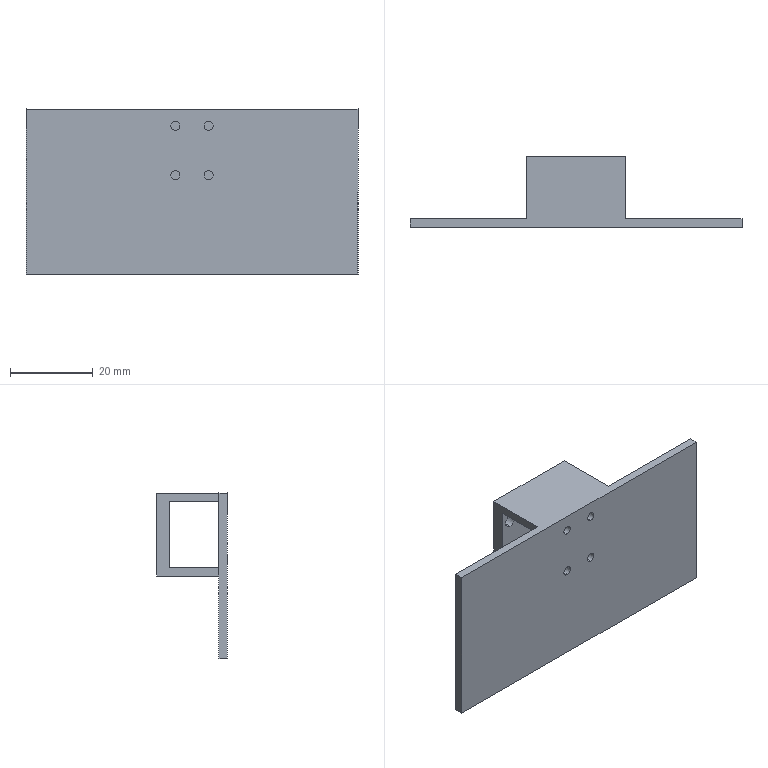Part | SolidWorks | features ICE 3, Extrusion 1 | 1 solid | 29 faces | box 80 x 17 x 40 mm | volume 8877 mm3 | cylinder 16 | plane 13 | commonest cylinder face diameters 2.2 x8 3 x8
STEP:
#1=CARTESIAN_POINT('',(9.5,14.,-3.));
#2=VERTEX_POINT('',#1);
#3=CARTESIAN_POINT('',(9.5,14.,-6.));
#4=VERTEX_POINT('',#3);
#5=CARTESIAN_POINT('',(9.5,14.,-4.5));
#6=DIRECTION('',(0.,-1.,0.));
#7=DIRECTION('',(0.,0.,-1.));
#8=AXIS2_PLACEMENT_3D('',#5,#6,#7);
#9=CIRCLE('',#8,1.5);
#10=EDGE_CURVE('',#2,#4,#9,.T.);
#11=ORIENTED_EDGE('',*,*,#10,.T.);
#12=CARTESIAN_POINT('',(9.5,17.,-6.));
#13=VERTEX_POINT('',#12);
#14=CARTESIAN_POINT('',(9.5,12.,-6.));
#15=DIRECTION('',(0.,1.,0.));
#16=VECTOR('',#15,1000.);
#17=LINE('',#14,#16);
#18=EDGE_CURVE('',#4,#13,#17,.T.);
#19=ORIENTED_EDGE('',*,*,#18,.T.);
#20=CARTESIAN_POINT('',(9.5,17.,-3.));
#21=VERTEX_POINT('',#20);
#22=CARTESIAN_POINT('',(9.5,17.,-4.5));
#23=DIRECTION('',(0.,1.,0.));
#24=DIRECTION('',(0.,0.,1.));
#25=AXIS2_PLACEMENT_3D('',#22,#23,#24);
#26=CIRCLE('',#25,1.5);
#27=EDGE_CURVE('',#13,#21,#26,.T.);
#28=ORIENTED_EDGE('',*,*,#27,.T.);
#29=CARTESIAN_POINT('',(9.5,12.,-3.));
#30=DIRECTION('',(0.,1.,0.));
#31=VECTOR('',#30,1000.);
#32=LINE('',#29,#31);
#33=EDGE_CURVE('',#2,#21,#32,.T.);
#34=ORIENTED_EDGE('',*,*,#33,.F.);
#35=EDGE_LOOP('',(#11,#19,#28,#34));
#36=FACE_OUTER_BOUND('',#35,.T.);
#37=CARTESIAN_POINT('',(9.5,12.,-4.5));
#38=DIRECTION('',(0.,1.,0.));
#39=DIRECTION('',(0.,0.,1.));
#40=AXIS2_PLACEMENT_3D('',#37,#38,#39);
#41=CYLINDRICAL_SURFACE('',#40,1.5);
#42=ADVANCED_FACE('',(#36),#41,.F.);
#43=CARTESIAN_POINT('',(-9.5,14.,-3.));
#44=VERTEX_POINT('',#43);
#45=CARTESIAN_POINT('',(-9.5,14.,-6.));
#46=VERTEX_POINT('',#45);
#47=CARTESIAN_POINT('',(-9.5,14.,-4.5));
#48=DIRECTION('',(0.,-1.,0.));
#49=DIRECTION('',(0.,0.,-1.));
#50=AXIS2_PLACEMENT_3D('',#47,#48,#49);
#51=CIRCLE('',#50,1.5);
#52=EDGE_CURVE('',#44,#46,#51,.T.);
#53=ORIENTED_EDGE('',*,*,#52,.T.);
#54=CARTESIAN_POINT('',(-9.5,17.,-6.));
#55=VERTEX_POINT('',#54);
#56=CARTESIAN_POINT('',(-9.5,12.,-6.));
#57=DIRECTION('',(0.,1.,0.));
#58=VECTOR('',#57,1000.);
#59=LINE('',#56,#58);
#60=EDGE_CURVE('',#46,#55,#59,.T.);
#61=ORIENTED_EDGE('',*,*,#60,.T.);
#62=CARTESIAN_POINT('',(-9.5,17.,-3.));
#63=VERTEX_POINT('',#62);
#64=CARTESIAN_POINT('',(-9.5,17.,-4.5));
#65=DIRECTION('',(0.,1.,0.));
#66=DIRECTION('',(0.,0.,1.));
#67=AXIS2_PLACEMENT_3D('',#64,#65,#66);
#68=CIRCLE('',#67,1.5);
#69=EDGE_CURVE('',#55,#63,#68,.T.);
#70=ORIENTED_EDGE('',*,*,#69,.T.);
#71=CARTESIAN_POINT('',(-9.5,12.,-3.));
#72=DIRECTION('',(0.,1.,0.));
#73=VECTOR('',#72,1000.);
#74=LINE('',#71,#73);
#75=EDGE_CURVE('',#44,#63,#74,.T.);
#76=ORIENTED_EDGE('',*,*,#75,.F.);
#77=EDGE_LOOP('',(#53,#61,#70,#76));
#78=FACE_OUTER_BOUND('',#77,.T.);
#79=CARTESIAN_POINT('',(-9.5,12.,-4.5));
#80=DIRECTION('',(0.,1.,0.));
#81=DIRECTION('',(0.,0.,1.));
#82=AXIS2_PLACEMENT_3D('',#79,#80,#81);
#83=CYLINDRICAL_SURFACE('',#82,1.5);
#84=ADVANCED_FACE('',(#78),#83,.F.);
#85=CARTESIAN_POINT('',(-9.5,14.,6.));
#86=VERTEX_POINT('',#85);
#87=CARTESIAN_POINT('',(-9.5,14.,3.));
#88=VERTEX_POINT('',#87);
#89=CARTESIAN_POINT('',(-9.5,14.,4.5));
#90=DIRECTION('',(0.,-1.,0.));
#91=DIRECTION('',(0.,0.,-1.));
#92=AXIS2_PLACEMENT_3D('',#89,#90,#91);
#93=CIRCLE('',#92,1.5);
#94=EDGE_CURVE('',#86,#88,#93,.T.);
#95=ORIENTED_EDGE('',*,*,#94,.T.);
#96=CARTESIAN_POINT('',(-9.5,17.,3.));
#97=VERTEX_POINT('',#96);
#98=CARTESIAN_POINT('',(-9.5,12.,3.));
#99=DIRECTION('',(0.,1.,0.));
#100=VECTOR('',#99,1000.);
#101=LINE('',#98,#100);
#102=EDGE_CURVE('',#88,#97,#101,.T.);
#103=ORIENTED_EDGE('',*,*,#102,.T.);
#104=CARTESIAN_POINT('',(-9.5,17.,6.));
#105=VERTEX_POINT('',#104);
#106=CARTESIAN_POINT('',(-9.5,17.,4.5));
#107=DIRECTION('',(0.,1.,0.));
#108=DIRECTION('',(0.,0.,1.));
#109=AXIS2_PLACEMENT_3D('',#106,#107,#108);
#110=CIRCLE('',#109,1.5);
#111=EDGE_CURVE('',#97,#105,#110,.T.);
#112=ORIENTED_EDGE('',*,*,#111,.T.);
#113=CARTESIAN_POINT('',(-9.5,12.,6.));
#114=DIRECTION('',(0.,1.,0.));
#115=VECTOR('',#114,1000.);
#116=LINE('',#113,#115);
#117=EDGE_CURVE('',#86,#105,#116,.T.);
#118=ORIENTED_EDGE('',*,*,#117,.F.);
#119=EDGE_LOOP('',(#95,#103,#112,#118));
#120=FACE_OUTER_BOUND('',#119,.T.);
#121=CARTESIAN_POINT('',(-9.5,12.,4.5));
#122=DIRECTION('',(0.,1.,0.));
#123=DIRECTION('',(0.,0.,1.));
#124=AXIS2_PLACEMENT_3D('',#121,#122,#123);
#125=CYLINDRICAL_SURFACE('',#124,1.5);
#126=ADVANCED_FACE('',(#120),#125,.F.);
#127=CARTESIAN_POINT('',(9.5,14.,6.));
#128=VERTEX_POINT('',#127);
#129=CARTESIAN_POINT('',(9.5,14.,3.));
#130=VERTEX_POINT('',#129);
#131=CARTESIAN_POINT('',(9.5,14.,4.5));
#132=DIRECTION('',(0.,-1.,0.));
#133=DIRECTION('',(0.,0.,-1.));
#134=AXIS2_PLACEMENT_3D('',#131,#132,#133);
#135=CIRCLE('',#134,1.5);
#136=EDGE_CURVE('',#128,#130,#135,.T.);
#137=ORIENTED_EDGE('',*,*,#136,.T.);
#138=CARTESIAN_POINT('',(9.5,17.,3.));
#139=VERTEX_POINT('',#138);
#140=CARTESIAN_POINT('',(9.5,12.,3.));
#141=DIRECTION('',(0.,1.,0.));
#142=VECTOR('',#141,1000.);
#143=LINE('',#140,#142);
#144=EDGE_CURVE('',#130,#139,#143,.T.);
#145=ORIENTED_EDGE('',*,*,#144,.T.);
#146=CARTESIAN_POINT('',(9.5,17.,6.));
#147=VERTEX_POINT('',#146);
#148=CARTESIAN_POINT('',(9.5,17.,4.5));
#149=DIRECTION('',(0.,1.,0.));
#150=DIRECTION('',(0.,0.,1.));
#151=AXIS2_PLACEMENT_3D('',#148,#149,#150);
#152=CIRCLE('',#151,1.5);
#153=EDGE_CURVE('',#139,#147,#152,.T.);
#154=ORIENTED_EDGE('',*,*,#153,.T.);
#155=CARTESIAN_POINT('',(9.5,12.,6.));
#156=DIRECTION('',(0.,1.,0.));
#157=VECTOR('',#156,1000.);
#158=LINE('',#155,#157);
#159=EDGE_CURVE('',#128,#147,#158,.T.);
#160=ORIENTED_EDGE('',*,*,#159,.F.);
#161=EDGE_LOOP('',(#137,#145,#154,#160));
#162=FACE_OUTER_BOUND('',#161,.T.);
#163=CARTESIAN_POINT('',(9.5,12.,4.5));
#164=DIRECTION('',(0.,1.,0.));
#165=DIRECTION('',(0.,0.,1.));
#166=AXIS2_PLACEMENT_3D('',#163,#164,#165);
#167=CYLINDRICAL_SURFACE('',#166,1.5);
#168=ADVANCED_FACE('',(#162),#167,.F.);
#169=CARTESIAN_POINT('',(4.,2.,4.9));
#170=VERTEX_POINT('',#169);
#171=CARTESIAN_POINT('',(4.,2.,7.1));
#172=VERTEX_POINT('',#171);
#173=CARTESIAN_POINT('',(4.,2.,6.));
#174=DIRECTION('',(0.,1.,0.));
#175=DIRECTION('',(0.,0.,1.));
#176=AXIS2_PLACEMENT_3D('',#173,#174,#175);
#177=CIRCLE('',#176,1.1);
#178=EDGE_CURVE('',#170,#172,#177,.T.);
#179=ORIENTED_EDGE('',*,*,#178,.T.);
#180=CARTESIAN_POINT('',(4.,0.,7.1));
#181=VERTEX_POINT('',#180);
#182=CARTESIAN_POINT('',(4.,2.,7.1));
#183=DIRECTION('',(0.,-1.,0.));
#184=VECTOR('',#183,1000.);
#185=LINE('',#182,#184);
#186=EDGE_CURVE('',#172,#181,#185,.T.);
#187=ORIENTED_EDGE('',*,*,#186,.T.);
#188=CARTESIAN_POINT('',(4.,0.,4.9));
#189=VERTEX_POINT('',#188);
#190=CARTESIAN_POINT('',(4.,0.,6.));
#191=DIRECTION('',(0.,1.,0.));
#192=DIRECTION('',(0.,0.,1.));
#193=AXIS2_PLACEMENT_3D('',#190,#191,#192);
#194=CIRCLE('',#193,1.1);
#195=EDGE_CURVE('',#189,#181,#194,.T.);
#196=ORIENTED_EDGE('',*,*,#195,.F.);
#197=CARTESIAN_POINT('',(4.,2.,4.9));
#198=DIRECTION('',(0.,-1.,0.));
#199=VECTOR('',#198,1000.);
#200=LINE('',#197,#199);
#201=EDGE_CURVE('',#170,#189,#200,.T.);
#202=ORIENTED_EDGE('',*,*,#201,.F.);
#203=EDGE_LOOP('',(#179,#187,#196,#202));
#204=FACE_OUTER_BOUND('',#203,.T.);
#205=CARTESIAN_POINT('',(4.,2.,6.));
#206=DIRECTION('',(0.,-1.,0.));
#207=DIRECTION('',(0.,0.,-1.));
#208=AXIS2_PLACEMENT_3D('',#205,#206,#207);
#209=CYLINDRICAL_SURFACE('',#208,1.1);
#210=ADVANCED_FACE('',(#204),#209,.F.);
#211=CARTESIAN_POINT('',(-4.,2.,4.9));
#212=VERTEX_POINT('',#211);
#213=CARTESIAN_POINT('',(-4.,2.,7.1));
#214=VERTEX_POINT('',#213);
#215=CARTESIAN_POINT('',(-4.,2.,6.));
#216=DIRECTION('',(0.,1.,0.));
#217=DIRECTION('',(0.,0.,1.));
#218=AXIS2_PLACEMENT_3D('',#215,#216,#217);
#219=CIRCLE('',#218,1.1);
#220=EDGE_CURVE('',#212,#214,#219,.T.);
#221=ORIENTED_EDGE('',*,*,#220,.T.);
#222=CARTESIAN_POINT('',(-4.,0.,7.1));
#223=VERTEX_POINT('',#222);
#224=CARTESIAN_POINT('',(-4.,2.,7.1));
#225=DIRECTION('',(0.,-1.,0.));
#226=VECTOR('',#225,1000.);
#227=LINE('',#224,#226);
#228=EDGE_CURVE('',#214,#223,#227,.T.);
#229=ORIENTED_EDGE('',*,*,#228,.T.);
#230=CARTESIAN_POINT('',(-4.,0.,4.9));
#231=VERTEX_POINT('',#230);
#232=CARTESIAN_POINT('',(-4.,0.,6.));
#233=DIRECTION('',(0.,1.,0.));
#234=DIRECTION('',(0.,0.,1.));
#235=AXIS2_PLACEMENT_3D('',#232,#233,#234);
#236=CIRCLE('',#235,1.1);
#237=EDGE_CURVE('',#231,#223,#236,.T.);
#238=ORIENTED_EDGE('',*,*,#237,.F.);
#239=CARTESIAN_POINT('',(-4.,2.,4.9));
#240=DIRECTION('',(0.,-1.,0.));
#241=VECTOR('',#240,1000.);
#242=LINE('',#239,#241);
#243=EDGE_CURVE('',#212,#231,#242,.T.);
#244=ORIENTED_EDGE('',*,*,#243,.F.);
#245=EDGE_LOOP('',(#221,#229,#238,#244));
#246=FACE_OUTER_BOUND('',#245,.T.);
#247=CARTESIAN_POINT('',(-4.,2.,6.));
#248=DIRECTION('',(0.,-1.,0.));
#249=DIRECTION('',(0.,0.,-1.));
#250=AXIS2_PLACEMENT_3D('',#247,#248,#249);
#251=CYLINDRICAL_SURFACE('',#250,1.1);
#252=ADVANCED_FACE('',(#246),#251,.F.);
#253=CARTESIAN_POINT('',(4.,2.,-7.1));
#254=VERTEX_POINT('',#253);
#255=CARTESIAN_POINT('',(4.,2.,-4.9));
#256=VERTEX_POINT('',#255);
#257=CARTESIAN_POINT('',(4.,2.,-6.));
#258=DIRECTION('',(0.,1.,0.));
#259=DIRECTION('',(0.,0.,1.));
#260=AXIS2_PLACEMENT_3D('',#257,#258,#259);
#261=CIRCLE('',#260,1.1);
#262=EDGE_CURVE('',#254,#256,#261,.T.);
#263=ORIENTED_EDGE('',*,*,#262,.T.);
#264=CARTESIAN_POINT('',(4.,0.,-4.9));
#265=VERTEX_POINT('',#264);
#266=CARTESIAN_POINT('',(4.,2.,-4.9));
#267=DIRECTION('',(0.,-1.,0.));
#268=VECTOR('',#267,1000.);
#269=LINE('',#266,#268);
#270=EDGE_CURVE('',#256,#265,#269,.T.);
#271=ORIENTED_EDGE('',*,*,#270,.T.);
#272=CARTESIAN_POINT('',(4.,0.,-7.1));
#273=VERTEX_POINT('',#272);
#274=CARTESIAN_POINT('',(4.,0.,-6.));
#275=DIRECTION('',(0.,1.,0.));
#276=DIRECTION('',(0.,0.,1.));
#277=AXIS2_PLACEMENT_3D('',#274,#275,#276);
#278=CIRCLE('',#277,1.1);
#279=EDGE_CURVE('',#273,#265,#278,.T.);
#280=ORIENTED_EDGE('',*,*,#279,.F.);
#281=CARTESIAN_POINT('',(4.,2.,-7.1));
#282=DIRECTION('',(0.,-1.,0.));
#283=VECTOR('',#282,1000.);
#284=LINE('',#281,#283);
#285=EDGE_CURVE('',#254,#273,#284,.T.);
#286=ORIENTED_EDGE('',*,*,#285,.F.);
#287=EDGE_LOOP('',(#263,#271,#280,#286));
#288=FACE_OUTER_BOUND('',#287,.T.);
#289=CARTESIAN_POINT('',(4.,2.,-6.));
#290=DIRECTION('',(0.,-1.,0.));
#291=DIRECTION('',(0.,0.,-1.));
#292=AXIS2_PLACEMENT_3D('',#289,#290,#291);
#293=CYLINDRICAL_SURFACE('',#292,1.1);
#294=ADVANCED_FACE('',(#288),#293,.F.);
#295=CARTESIAN_POINT('',(-4.,2.,-7.1));
#296=VERTEX_POINT('',#295);
#297=CARTESIAN_POINT('',(-4.,2.,-4.9));
#298=VERTEX_POINT('',#297);
#299=CARTESIAN_POINT('',(-4.,2.,-6.));
#300=DIRECTION('',(0.,1.,0.));
#301=DIRECTION('',(0.,0.,1.));
#302=AXIS2_PLACEMENT_3D('',#299,#300,#301);
#303=CIRCLE('',#302,1.1);
#304=EDGE_CURVE('',#296,#298,#303,.T.);
#305=ORIENTED_EDGE('',*,*,#304,.T.);
#306=CARTESIAN_POINT('',(-4.,0.,-4.9));
#307=VERTEX_POINT('',#306);
#308=CARTESIAN_POINT('',(-4.,2.,-4.9));
#309=DIRECTION('',(0.,-1.,0.));
#310=VECTOR('',#309,1000.);
#311=LINE('',#308,#310);
#312=EDGE_CURVE('',#298,#307,#311,.T.);
#313=ORIENTED_EDGE('',*,*,#312,.T.);
#314=CARTESIAN_POINT('',(-4.,0.,-7.1));
#315=VERTEX_POINT('',#314);
#316=CARTESIAN_POINT('',(-4.,0.,-6.));
#317=DIRECTION('',(0.,1.,0.));
#318=DIRECTION('',(0.,0.,1.));
#319=AXIS2_PLACEMENT_3D('',#316,#317,#318);
#320=CIRCLE('',#319,1.1);
#321=EDGE_CURVE('',#315,#307,#320,.T.);
#322=ORIENTED_EDGE('',*,*,#321,.F.);
#323=CARTESIAN_POINT('',(-4.,2.,-7.1));
#324=DIRECTION('',(0.,-1.,0.));
#325=VECTOR('',#324,1000.);
#326=LINE('',#323,#325);
#327=EDGE_CURVE('',#296,#315,#326,.T.);
#328=ORIENTED_EDGE('',*,*,#327,.F.);
#329=EDGE_LOOP('',(#305,#313,#322,#328));
#330=FACE_OUTER_BOUND('',#329,.T.);
#331=CARTESIAN_POINT('',(-4.,2.,-6.));
#332=DIRECTION('',(0.,-1.,0.));
#333=DIRECTION('',(0.,0.,-1.));
#334=AXIS2_PLACEMENT_3D('',#331,#332,#333);
#335=CYLINDRICAL_SURFACE('',#334,1.1);
#336=ADVANCED_FACE('',(#330),#335,.F.);
#337=CARTESIAN_POINT('',(12.,2.,-10.));
#338=VERTEX_POINT('',#337);
#339=CARTESIAN_POINT('',(-12.,2.,-10.));
#340=VERTEX_POINT('',#339);
#341=CARTESIAN_POINT('',(40.,2.,-10.));
#342=DIRECTION('',(-1.,0.,0.));
#343=VECTOR('',#342,1000.);
#344=LINE('',#341,#343);
#345=EDGE_CURVE('',#338,#340,#344,.T.);
#346=ORIENTED_EDGE('',*,*,#345,.F.);
#347=CARTESIAN_POINT('',(12.,2.,-8.));
#348=VERTEX_POINT('',#347);
#349=CARTESIAN_POINT('',(12.,2.,-10.));
#350=DIRECTION('',(0.,0.,-1.));
#351=VECTOR('',#350,1000.);
#352=LINE('',#349,#351);
#353=EDGE_CURVE('',#348,#338,#352,.T.);
#354=ORIENTED_EDGE('',*,*,#353,.F.);
#355=CARTESIAN_POINT('',(-12.,2.,-8.));
#356=VERTEX_POINT('',#355);
#357=CARTESIAN_POINT('',(-12.,2.,-8.));
#358=DIRECTION('',(1.,0.,0.));
#359=VECTOR('',#358,1000.);
#360=LINE('',#357,#359);
#361=EDGE_CURVE('',#356,#348,#360,.T.);
#362=ORIENTED_EDGE('',*,*,#361,.F.);
#363=CARTESIAN_POINT('',(-12.,2.,-10.));
#364=DIRECTION('',(0.,0.,-1.));
#365=VECTOR('',#364,1000.);
#366=LINE('',#363,#365);
#367=EDGE_CURVE('',#356,#340,#366,.T.);
#368=ORIENTED_EDGE('',*,*,#367,.T.);
#369=EDGE_LOOP('',(#346,#354,#362,#368));
#370=FACE_BOUND('',#369,.T.);
#371=CARTESIAN_POINT('',(-40.,2.,10.));
#372=VERTEX_POINT('',#371);
#373=CARTESIAN_POINT('',(-12.,2.,10.));
#374=VERTEX_POINT('',#373);
#375=CARTESIAN_POINT('',(-40.,2.,10.));
#376=DIRECTION('',(1.,0.,0.));
#377=VECTOR('',#376,1000.);
#378=LINE('',#375,#377);
#379=EDGE_CURVE('',#372,#374,#378,.T.);
#380=ORIENTED_EDGE('',*,*,#379,.T.);
#381=CARTESIAN_POINT('',(-12.,2.,8.));
#382=VERTEX_POINT('',#381);
#383=CARTESIAN_POINT('',(-12.,2.,10.));
#384=DIRECTION('',(0.,0.,-1.));
#385=VECTOR('',#384,1000.);
#386=LINE('',#383,#385);
#387=EDGE_CURVE('',#374,#382,#386,.T.);
#388=ORIENTED_EDGE('',*,*,#387,.T.);
#389=CARTESIAN_POINT('',(12.,2.,8.));
#390=VERTEX_POINT('',#389);
#391=CARTESIAN_POINT('',(-12.,2.,8.));
#392=DIRECTION('',(1.,0.,0.));
#393=VECTOR('',#392,1000.);
#394=LINE('',#391,#393);
#395=EDGE_CURVE('',#382,#390,#394,.T.);
#396=ORIENTED_EDGE('',*,*,#395,.T.);
#397=CARTESIAN_POINT('',(12.,2.,10.));
#398=VERTEX_POINT('',#397);
#399=CARTESIAN_POINT('',(12.,2.,10.));
#400=DIRECTION('',(0.,0.,-1.));
#401=VECTOR('',#400,1000.);
#402=LINE('',#399,#401);
#403=EDGE_CURVE('',#398,#390,#402,.T.);
#404=ORIENTED_EDGE('',*,*,#403,.F.);
#405=CARTESIAN_POINT('',(40.,2.,10.));
#406=VERTEX_POINT('',#405);
#407=CARTESIAN_POINT('',(-40.,2.,10.));
#408=DIRECTION('',(1.,0.,0.));
#409=VECTOR('',#408,1000.);
#410=LINE('',#407,#409);
#411=EDGE_CURVE('',#398,#406,#410,.T.);
#412=ORIENTED_EDGE('',*,*,#411,.T.);
#413=CARTESIAN_POINT('',(40.,2.,-30.));
#414=VERTEX_POINT('',#413);
#415=CARTESIAN_POINT('',(40.,2.,10.));
#416=DIRECTION('',(0.,0.,-1.));
#417=VECTOR('',#416,1000.);
#418=LINE('',#415,#417);
#419=EDGE_CURVE('',#406,#414,#418,.T.);
#420=ORIENTED_EDGE('',*,*,#419,.T.);
#421=CARTESIAN_POINT('',(-40.,2.,-30.));
#422=VERTEX_POINT('',#421);
#423=CARTESIAN_POINT('',(40.,2.,-30.));
#424=DIRECTION('',(-1.,0.,0.));
#425=VECTOR('',#424,1000.);
#426=LINE('',#423,#425);
#427=EDGE_CURVE('',#414,#422,#426,.T.);
#428=ORIENTED_EDGE('',*,*,#427,.T.);
#429=CARTESIAN_POINT('',(-40.,2.,10.));
#430=DIRECTION('',(0.,0.,1.));
#431=VECTOR('',#430,1000.);
#432=LINE('',#429,#431);
#433=EDGE_CURVE('',#422,#372,#432,.T.);
#434=ORIENTED_EDGE('',*,*,#433,.T.);
#435=EDGE_LOOP('',(#380,#388,#396,#404,#412,#420,#428,#434));
#436=FACE_OUTER_BOUND('',#435,.T.);
#437=ORIENTED_EDGE('',*,*,#304,.F.);
#438=CARTESIAN_POINT('',(-4.,2.,-6.));
#439=DIRECTION('',(0.,1.,0.));
#440=DIRECTION('',(0.,0.,1.));
#441=AXIS2_PLACEMENT_3D('',#438,#439,#440);
#442=CIRCLE('',#441,1.1);
#443=EDGE_CURVE('',#298,#296,#442,.T.);
#444=ORIENTED_EDGE('',*,*,#443,.F.);
#445=EDGE_LOOP('',(#437,#444));
#446=FACE_BOUND('',#445,.T.);
#447=ORIENTED_EDGE('',*,*,#262,.F.);
#448=CARTESIAN_POINT('',(4.,2.,-6.));
#449=DIRECTION('',(0.,1.,0.));
#450=DIRECTION('',(0.,0.,1.));
#451=AXIS2_PLACEMENT_3D('',#448,#449,#450);
#452=CIRCLE('',#451,1.1);
#453=EDGE_CURVE('',#256,#254,#452,.T.);
#454=ORIENTED_EDGE('',*,*,#453,.F.);
#455=EDGE_LOOP('',(#447,#454));
#456=FACE_BOUND('',#455,.T.);
#457=ORIENTED_EDGE('',*,*,#220,.F.);
#458=CARTESIAN_POINT('',(-4.,2.,6.));
#459=DIRECTION('',(0.,1.,0.));
#460=DIRECTION('',(0.,0.,1.));
#461=AXIS2_PLACEMENT_3D('',#458,#459,#460);
#462=CIRCLE('',#461,1.1);
#463=EDGE_CURVE('',#214,#212,#462,.T.);
#464=ORIENTED_EDGE('',*,*,#463,.F.);
#465=EDGE_LOOP('',(#457,#464));
#466=FACE_BOUND('',#465,.T.);
#467=ORIENTED_EDGE('',*,*,#178,.F.);
#468=CARTESIAN_POINT('',(4.,2.,6.));
#469=DIRECTION('',(0.,1.,0.));
#470=DIRECTION('',(0.,0.,1.));
#471=AXIS2_PLACEMENT_3D('',#468,#469,#470);
#472=CIRCLE('',#471,1.1);
#473=EDGE_CURVE('',#172,#170,#472,.T.);
#474=ORIENTED_EDGE('',*,*,#473,.F.);
#475=EDGE_LOOP('',(#467,#474));
#476=FACE_BOUND('',#475,.T.);
#477=CARTESIAN_POINT('',(0.,2.,0.));
#478=DIRECTION('',(0.,-1.,0.));
#479=DIRECTION('',(0.,0.,-1.));
#480=AXIS2_PLACEMENT_3D('',#477,#478,#479);
#481=PLANE('',#480);
#482=ADVANCED_FACE('',(#370,#436,#446,#456,#466,#476),#481,.F.);
#483=ORIENTED_EDGE('',*,*,#237,.T.);
#484=CARTESIAN_POINT('',(-4.,0.,6.));
#485=DIRECTION('',(0.,1.,0.));
#486=DIRECTION('',(0.,0.,1.));
#487=AXIS2_PLACEMENT_3D('',#484,#485,#486);
#488=CIRCLE('',#487,1.1);
#489=EDGE_CURVE('',#223,#231,#488,.T.);
#490=ORIENTED_EDGE('',*,*,#489,.T.);
#491=EDGE_LOOP('',(#483,#490));
#492=FACE_BOUND('',#491,.T.);
#493=ORIENTED_EDGE('',*,*,#321,.T.);
#494=CARTESIAN_POINT('',(-4.,0.,-6.));
#495=DIRECTION('',(0.,1.,0.));
#496=DIRECTION('',(0.,0.,1.));
#497=AXIS2_PLACEMENT_3D('',#494,#495,#496);
#498=CIRCLE('',#497,1.1);
#499=EDGE_CURVE('',#307,#315,#498,.T.);
#500=ORIENTED_EDGE('',*,*,#499,.T.);
#501=EDGE_LOOP('',(#493,#500));
#502=FACE_BOUND('',#501,.T.);
#503=CARTESIAN_POINT('',(40.,0.,10.));
#504=VERTEX_POINT('',#503);
#505=CARTESIAN_POINT('',(40.,0.,-30.));
#506=VERTEX_POINT('',#505);
#507=CARTESIAN_POINT('',(40.,0.,10.));
#508=DIRECTION('',(0.,0.,-1.));
#509=VECTOR('',#508,1000.);
#510=LINE('',#507,#509);
#511=EDGE_CURVE('',#504,#506,#510,.T.);
#512=ORIENTED_EDGE('',*,*,#511,.F.);
#513=CARTESIAN_POINT('',(-40.,0.,10.));
#514=VERTEX_POINT('',#513);
#515=CARTESIAN_POINT('',(-40.,0.,10.));
#516=DIRECTION('',(1.,0.,0.));
#517=VECTOR('',#516,1000.);
#518=LINE('',#515,#517);
#519=EDGE_CURVE('',#514,#504,#518,.T.);
#520=ORIENTED_EDGE('',*,*,#519,.F.);
#521=CARTESIAN_POINT('',(-40.,0.,-30.));
#522=VERTEX_POINT('',#521);
#523=CARTESIAN_POINT('',(-40.,0.,10.));
#524=DIRECTION('',(0.,0.,1.));
#525=VECTOR('',#524,1000.);
#526=LINE('',#523,#525);
#527=EDGE_CURVE('',#522,#514,#526,.T.);
#528=ORIENTED_EDGE('',*,*,#527,.F.);
#529=CARTESIAN_POINT('',(40.,0.,-30.));
#530=DIRECTION('',(1.,0.,0.));
#531=VECTOR('',#530,1000.);
#532=LINE('',#529,#531);
#533=EDGE_CURVE('',#522,#506,#532,.T.);
#534=ORIENTED_EDGE('',*,*,#533,.T.);
#535=EDGE_LOOP('',(#512,#520,#528,#534));
#536=FACE_OUTER_BOUND('',#535,.T.);
#537=ORIENTED_EDGE('',*,*,#279,.T.);
#538=CARTESIAN_POINT('',(4.,0.,-6.));
#539=DIRECTION('',(0.,1.,0.));
#540=DIRECTION('',(0.,0.,1.));
#541=AXIS2_PLACEMENT_3D('',#538,#539,#540);
#542=CIRCLE('',#541,1.1);
#543=EDGE_CURVE('',#265,#273,#542,.T.);
#544=ORIENTED_EDGE('',*,*,#543,.T.);
#545=EDGE_LOOP('',(#537,#544));
#546=FACE_BOUND('',#545,.T.);
#547=ORIENTED_EDGE('',*,*,#195,.T.);
#548=CARTESIAN_POINT('',(4.,0.,6.));
#549=DIRECTION('',(0.,1.,0.));
#550=DIRECTION('',(0.,0.,1.));
#551=AXIS2_PLACEMENT_3D('',#548,#549,#550);
#552=CIRCLE('',#551,1.1);
#553=EDGE_CURVE('',#181,#189,#552,.T.);
#554=ORIENTED_EDGE('',*,*,#553,.T.);
#555=EDGE_LOOP('',(#547,#554));
#556=FACE_BOUND('',#555,.T.);
#557=CARTESIAN_POINT('',(0.,0.,0.));
#558=DIRECTION('',(0.,-1.,0.));
#559=DIRECTION('',(0.,0.,-1.));
#560=AXIS2_PLACEMENT_3D('',#557,#558,#559);
#561=PLANE('',#560);
#562=ADVANCED_FACE('',(#492,#502,#536,#546,#556),#561,.T.);
#563=ORIENTED_EDGE('',*,*,#511,.T.);
#564=CARTESIAN_POINT('',(40.,0.,-30.));
#565=DIRECTION('',(0.,1.,0.));
#566=VECTOR('',#565,1000.);
#567=LINE('',#564,#566);
#568=EDGE_CURVE('',#506,#414,#567,.T.);
#569=ORIENTED_EDGE('',*,*,#568,.T.);
#570=ORIENTED_EDGE('',*,*,#419,.F.);
#571=CARTESIAN_POINT('',(40.,2.,10.));
#572=DIRECTION('',(0.,-1.,0.));
#573=VECTOR('',#572,1000.);
#574=LINE('',#571,#573);
#575=EDGE_CURVE('',#406,#504,#574,.T.);
#576=ORIENTED_EDGE('',*,*,#575,.T.);
#577=EDGE_LOOP('',(#563,#569,#570,#576));
#578=FACE_OUTER_BOUND('',#577,.T.);
#579=CARTESIAN_POINT('',(40.,2.,10.));
#580=DIRECTION('',(-1.,0.,0.));
#581=DIRECTION('',(0.,0.,1.));
#582=AXIS2_PLACEMENT_3D('',#579,#580,#581);
#583=PLANE('',#582);
#584=ADVANCED_FACE('',(#578),#583,.F.);
#585=CARTESIAN_POINT('',(12.,17.,-10.));
#586=VERTEX_POINT('',#585);
#587=CARTESIAN_POINT('',(12.,13.783,-10.));
#588=DIRECTION('',(0.,1.,0.));
#589=VECTOR('',#588,1000.);
#590=LINE('',#587,#589);
#591=EDGE_CURVE('',#338,#586,#590,.T.);
#592=ORIENTED_EDGE('',*,*,#591,.F.);
#593=ORIENTED_EDGE('',*,*,#345,.T.);
#594=CARTESIAN_POINT('',(-12.,17.,-10.));
#595=VERTEX_POINT('',#594);
#596=CARTESIAN_POINT('',(-12.,2.,-10.));
#597=DIRECTION('',(0.,1.,0.));
#598=VECTOR('',#597,1000.);
#599=LINE('',#596,#598);
#600=EDGE_CURVE('',#340,#595,#599,.T.);
#601=ORIENTED_EDGE('',*,*,#600,.T.);
#602=CARTESIAN_POINT('',(-12.,17.,-10.));
#603=DIRECTION('',(1.,0.,0.));
#604=VECTOR('',#603,1000.);
#605=LINE('',#602,#604);
#606=EDGE_CURVE('',#595,#586,#605,.T.);
#607=ORIENTED_EDGE('',*,*,#606,.T.);
#608=EDGE_LOOP('',(#592,#593,#601,#607));
#609=FACE_OUTER_BOUND('',#608,.T.);
#610=CARTESIAN_POINT('',(-40.,2.,-10.));
#611=DIRECTION('',(0.,0.,1.));
#612=DIRECTION('',(1.,0.,0.));
#613=AXIS2_PLACEMENT_3D('',#610,#611,#612);
#614=PLANE('',#613);
#615=ADVANCED_FACE('',(#609),#614,.F.);
#616=ORIENTED_EDGE('',*,*,#527,.T.);
#617=CARTESIAN_POINT('',(-40.,2.,10.));
#618=DIRECTION('',(0.,-1.,0.));
#619=VECTOR('',#618,1000.);
#620=LINE('',#617,#619);
#621=EDGE_CURVE('',#372,#514,#620,.T.);
#622=ORIENTED_EDGE('',*,*,#621,.F.);
#623=ORIENTED_EDGE('',*,*,#433,.F.);
#624=CARTESIAN_POINT('',(-40.,0.,-30.));
#625=DIRECTION('',(0.,-1.,0.));
#626=VECTOR('',#625,1000.);
#627=LINE('',#624,#626);
#628=EDGE_CURVE('',#422,#522,#627,.T.);
#629=ORIENTED_EDGE('',*,*,#628,.T.);
#630=EDGE_LOOP('',(#616,#622,#623,#629));
#631=FACE_OUTER_BOUND('',#630,.T.);
#632=CARTESIAN_POINT('',(-40.,2.,10.));
#633=DIRECTION('',(1.,0.,0.));
#634=DIRECTION('',(0.,0.,-1.));
#635=AXIS2_PLACEMENT_3D('',#632,#633,#634);
#636=PLANE('',#635);
#637=ADVANCED_FACE('',(#631),#636,.F.);
#638=ORIENTED_EDGE('',*,*,#519,.T.);
#639=ORIENTED_EDGE('',*,*,#575,.F.);
#640=ORIENTED_EDGE('',*,*,#411,.F.);
#641=CARTESIAN_POINT('',(12.,17.,10.));
#642=VERTEX_POINT('',#641);
#643=CARTESIAN_POINT('',(12.,13.783,10.));
#644=DIRECTION('',(0.,-1.,0.));
#645=VECTOR('',#644,1000.);
#646=LINE('',#643,#645);
#647=EDGE_CURVE('',#642,#398,#646,.T.);
#648=ORIENTED_EDGE('',*,*,#647,.F.);
#649=CARTESIAN_POINT('',(-12.,17.,10.));
#650=VERTEX_POINT('',#649);
#651=CARTESIAN_POINT('',(-12.,17.,10.));
#652=DIRECTION('',(1.,0.,0.));
#653=VECTOR('',#652,1000.);
#654=LINE('',#651,#653);
#655=EDGE_CURVE('',#650,#642,#654,.T.);
#656=ORIENTED_EDGE('',*,*,#655,.F.);
#657=CARTESIAN_POINT('',(-12.,2.,10.));
#658=DIRECTION('',(0.,-1.,0.));
#659=VECTOR('',#658,1000.);
#660=LINE('',#657,#659);
#661=EDGE_CURVE('',#650,#374,#660,.T.);
#662=ORIENTED_EDGE('',*,*,#661,.T.);
#663=ORIENTED_EDGE('',*,*,#379,.F.);
#664=ORIENTED_EDGE('',*,*,#621,.T.);
#665=EDGE_LOOP('',(#638,#639,#640,#648,#656,#662,#663,#664));
#666=FACE_OUTER_BOUND('',#665,.T.);
#667=CARTESIAN_POINT('',(-40.,2.,10.));
#668=DIRECTION('',(0.,0.,-1.));
#669=DIRECTION('',(-1.,0.,0.));
#670=AXIS2_PLACEMENT_3D('',#667,#668,#669);
#671=PLANE('',#670);
#672=ADVANCED_FACE('',(#666),#671,.F.);
#673=ORIENTED_EDGE('',*,*,#312,.F.);
#674=ORIENTED_EDGE('',*,*,#443,.T.);
#675=ORIENTED_EDGE('',*,*,#327,.T.);
#676=ORIENTED_EDGE('',*,*,#499,.F.);
#677=EDGE_LOOP('',(#673,#674,#675,#676));
#678=FACE_OUTER_BOUND('',#677,.T.);
#679=CARTESIAN_POINT('',(-4.,2.,-6.));
#680=DIRECTION('',(0.,-1.,0.));
#681=DIRECTION('',(0.,0.,-1.));
#682=AXIS2_PLACEMENT_3D('',#679,#680,#681);
#683=CYLINDRICAL_SURFACE('',#682,1.1);
#684=ADVANCED_FACE('',(#678),#683,.F.);
#685=ORIENTED_EDGE('',*,*,#270,.F.);
#686=ORIENTED_EDGE('',*,*,#453,.T.);
#687=ORIENTED_EDGE('',*,*,#285,.T.);
#688=ORIENTED_EDGE('',*,*,#543,.F.);
#689=EDGE_LOOP('',(#685,#686,#687,#688));
#690=FACE_OUTER_BOUND('',#689,.T.);
#691=CARTESIAN_POINT('',(4.,2.,-6.));
#692=DIRECTION('',(0.,-1.,0.));
#693=DIRECTION('',(0.,0.,-1.));
#694=AXIS2_PLACEMENT_3D('',#691,#692,#693);
#695=CYLINDRICAL_SURFACE('',#694,1.1);
#696=ADVANCED_FACE('',(#690),#695,.F.);
#697=ORIENTED_EDGE('',*,*,#228,.F.);
#698=ORIENTED_EDGE('',*,*,#463,.T.);
#699=ORIENTED_EDGE('',*,*,#243,.T.);
#700=ORIENTED_EDGE('',*,*,#489,.F.);
#701=EDGE_LOOP('',(#697,#698,#699,#700));
#702=FACE_OUTER_BOUND('',#701,.T.);
#703=CARTESIAN_POINT('',(-4.,2.,6.));
#704=DIRECTION('',(0.,-1.,0.));
#705=DIRECTION('',(0.,0.,-1.));
#706=AXIS2_PLACEMENT_3D('',#703,#704,#705);
#707=CYLINDRICAL_SURFACE('',#706,1.1);
#708=ADVANCED_FACE('',(#702),#707,.F.);
#709=ORIENTED_EDGE('',*,*,#186,.F.);
#710=ORIENTED_EDGE('',*,*,#473,.T.);
#711=ORIENTED_EDGE('',*,*,#201,.T.);
#712=ORIENTED_EDGE('',*,*,#553,.F.);
#713=EDGE_LOOP('',(#709,#710,#711,#712));
#714=FACE_OUTER_BOUND('',#713,.T.);
#715=CARTESIAN_POINT('',(4.,2.,6.));
#716=DIRECTION('',(0.,-1.,0.));
#717=DIRECTION('',(0.,0.,-1.));
#718=AXIS2_PLACEMENT_3D('',#715,#716,#717);
#719=CYLINDRICAL_SURFACE('',#718,1.1);
#720=ADVANCED_FACE('',(#714),#719,.F.);
#721=CARTESIAN_POINT('',(9.5,17.,-4.5));
#722=DIRECTION('',(0.,1.,0.));
#723=DIRECTION('',(0.,0.,1.));
#724=AXIS2_PLACEMENT_3D('',#721,#722,#723);
#725=CIRCLE('',#724,1.5);
#726=EDGE_CURVE('',#21,#13,#725,.T.);
#727=ORIENTED_EDGE('',*,*,#726,.F.);
#728=ORIENTED_EDGE('',*,*,#27,.F.);
#729=EDGE_LOOP('',(#727,#728));
#730=FACE_BOUND('',#729,.T.);
#731=CARTESIAN_POINT('',(-9.5,17.,-4.5));
#732=DIRECTION('',(0.,1.,0.));
#733=DIRECTION('',(0.,0.,1.));
#734=AXIS2_PLACEMENT_3D('',#731,#732,#733);
#735=CIRCLE('',#734,1.5);
#736=EDGE_CURVE('',#63,#55,#735,.T.);
#737=ORIENTED_EDGE('',*,*,#736,.F.);
#738=ORIENTED_EDGE('',*,*,#69,.F.);
#739=EDGE_LOOP('',(#737,#738));
#740=FACE_BOUND('',#739,.T.);
#741=CARTESIAN_POINT('',(-9.5,17.,4.5));
#742=DIRECTION('',(0.,1.,0.));
#743=DIRECTION('',(0.,0.,1.));
#744=AXIS2_PLACEMENT_3D('',#741,#742,#743);
#745=CIRCLE('',#744,1.5);
#746=EDGE_CURVE('',#105,#97,#745,.T.);
#747=ORIENTED_EDGE('',*,*,#746,.F.);
#748=ORIENTED_EDGE('',*,*,#111,.F.);
#749=EDGE_LOOP('',(#747,#748));
#750=FACE_BOUND('',#749,.T.);
#751=CARTESIAN_POINT('',(9.5,17.,4.5));
#752=DIRECTION('',(0.,1.,0.));
#753=DIRECTION('',(0.,0.,1.));
#754=AXIS2_PLACEMENT_3D('',#751,#752,#753);
#755=CIRCLE('',#754,1.5);
#756=EDGE_CURVE('',#147,#139,#755,.T.);
#757=ORIENTED_EDGE('',*,*,#756,.F.);
#758=ORIENTED_EDGE('',*,*,#153,.F.);
#759=EDGE_LOOP('',(#757,#758));
#760=FACE_BOUND('',#759,.T.);
#761=CARTESIAN_POINT('',(12.,17.,10.));
#762=DIRECTION('',(0.,0.,1.));
#763=VECTOR('',#762,1000.);
#764=LINE('',#761,#763);
#765=EDGE_CURVE('',#586,#642,#764,.T.);
#766=ORIENTED_EDGE('',*,*,#765,.F.);
#767=ORIENTED_EDGE('',*,*,#606,.F.);
#768=CARTESIAN_POINT('',(-12.,17.,10.));
#769=DIRECTION('',(0.,0.,1.));
#770=VECTOR('',#769,1000.);
#771=LINE('',#768,#770);
#772=EDGE_CURVE('',#595,#650,#771,.T.);
#773=ORIENTED_EDGE('',*,*,#772,.T.);
#774=ORIENTED_EDGE('',*,*,#655,.T.);
#775=EDGE_LOOP('',(#766,#767,#773,#774));
#776=FACE_OUTER_BOUND('',#775,.T.);
#777=CARTESIAN_POINT('',(-12.,17.,10.));
#778=DIRECTION('',(0.,1.,0.));
#779=DIRECTION('',(0.,0.,1.));
#780=AXIS2_PLACEMENT_3D('',#777,#778,#779);
#781=PLANE('',#780);
#782=ADVANCED_FACE('',(#730,#740,#750,#760,#776),#781,.T.);
#783=CARTESIAN_POINT('',(12.,14.,-8.));
#784=VERTEX_POINT('',#783);
#785=CARTESIAN_POINT('',(12.,2.,-8.));
#786=DIRECTION('',(0.,-1.,0.));
#787=VECTOR('',#786,1000.);
#788=LINE('',#785,#787);
#789=EDGE_CURVE('',#784,#348,#788,.T.);
#790=ORIENTED_EDGE('',*,*,#789,.F.);
#791=CARTESIAN_POINT('',(-12.,14.,-8.));
#792=VERTEX_POINT('',#791);
#793=CARTESIAN_POINT('',(-12.,14.,-8.));
#794=DIRECTION('',(1.,0.,0.));
#795=VECTOR('',#794,1000.);
#796=LINE('',#793,#795);
#797=EDGE_CURVE('',#792,#784,#796,.T.);
#798=ORIENTED_EDGE('',*,*,#797,.F.);
#799=CARTESIAN_POINT('',(-12.,2.,-8.));
#800=DIRECTION('',(0.,-1.,0.));
#801=VECTOR('',#800,1000.);
#802=LINE('',#799,#801);
#803=EDGE_CURVE('',#792,#356,#802,.T.);
#804=ORIENTED_EDGE('',*,*,#803,.T.);
#805=ORIENTED_EDGE('',*,*,#361,.T.);
#806=EDGE_LOOP('',(#790,#798,#804,#805));
#807=FACE_OUTER_BOUND('',#806,.T.);
#808=CARTESIAN_POINT('',(-12.,2.,-8.));
#809=DIRECTION('',(0.,0.,1.));
#810=DIRECTION('',(1.,0.,0.));
#811=AXIS2_PLACEMENT_3D('',#808,#809,#810);
#812=PLANE('',#811);
#813=ADVANCED_FACE('',(#807),#812,.T.);
#814=ORIENTED_EDGE('',*,*,#10,.F.);
#815=CARTESIAN_POINT('',(9.5,14.,-4.5));
#816=DIRECTION('',(0.,-1.,0.));
#817=DIRECTION('',(0.,0.,-1.));
#818=AXIS2_PLACEMENT_3D('',#815,#816,#817);
#819=CIRCLE('',#818,1.5);
#820=EDGE_CURVE('',#4,#2,#819,.T.);
#821=ORIENTED_EDGE('',*,*,#820,.F.);
#822=EDGE_LOOP('',(#814,#821));
#823=FACE_BOUND('',#822,.T.);
#824=ORIENTED_EDGE('',*,*,#52,.F.);
#825=CARTESIAN_POINT('',(-9.5,14.,-4.5));
#826=DIRECTION('',(0.,-1.,0.));
#827=DIRECTION('',(0.,0.,-1.));
#828=AXIS2_PLACEMENT_3D('',#825,#826,#827);
#829=CIRCLE('',#828,1.5);
#830=EDGE_CURVE('',#46,#44,#829,.T.);
#831=ORIENTED_EDGE('',*,*,#830,.F.);
#832=EDGE_LOOP('',(#824,#831));
#833=FACE_BOUND('',#832,.T.);
#834=ORIENTED_EDGE('',*,*,#94,.F.);
#835=CARTESIAN_POINT('',(-9.5,14.,4.5));
#836=DIRECTION('',(0.,-1.,0.));
#837=DIRECTION('',(0.,0.,-1.));
#838=AXIS2_PLACEMENT_3D('',#835,#836,#837);
#839=CIRCLE('',#838,1.5);
#840=EDGE_CURVE('',#88,#86,#839,.T.);
#841=ORIENTED_EDGE('',*,*,#840,.F.);
#842=EDGE_LOOP('',(#834,#841));
#843=FACE_BOUND('',#842,.T.);
#844=ORIENTED_EDGE('',*,*,#136,.F.);
#845=CARTESIAN_POINT('',(9.5,14.,4.5));
#846=DIRECTION('',(0.,-1.,0.));
#847=DIRECTION('',(0.,0.,-1.));
#848=AXIS2_PLACEMENT_3D('',#845,#846,#847);
#849=CIRCLE('',#848,1.5);
#850=EDGE_CURVE('',#130,#128,#849,.T.);
#851=ORIENTED_EDGE('',*,*,#850,.F.);
#852=EDGE_LOOP('',(#844,#851));
#853=FACE_BOUND('',#852,.T.);
#854=CARTESIAN_POINT('',(12.,14.,8.));
#855=VERTEX_POINT('',#854);
#856=CARTESIAN_POINT('',(12.,14.,8.));
#857=DIRECTION('',(0.,0.,-1.));
#858=VECTOR('',#857,1000.);
#859=LINE('',#856,#858);
#860=EDGE_CURVE('',#855,#784,#859,.T.);
#861=ORIENTED_EDGE('',*,*,#860,.F.);
#862=CARTESIAN_POINT('',(-12.,14.,8.));
#863=VERTEX_POINT('',#862);
#864=CARTESIAN_POINT('',(-12.,14.,8.));
#865=DIRECTION('',(1.,0.,0.));
#866=VECTOR('',#865,1000.);
#867=LINE('',#864,#866);
#868=EDGE_CURVE('',#863,#855,#867,.T.);
#869=ORIENTED_EDGE('',*,*,#868,.F.);
#870=CARTESIAN_POINT('',(-12.,14.,8.));
#871=DIRECTION('',(0.,0.,-1.));
#872=VECTOR('',#871,1000.);
#873=LINE('',#870,#872);
#874=EDGE_CURVE('',#863,#792,#873,.T.);
#875=ORIENTED_EDGE('',*,*,#874,.T.);
#876=ORIENTED_EDGE('',*,*,#797,.T.);
#877=EDGE_LOOP('',(#861,#869,#875,#876));
#878=FACE_OUTER_BOUND('',#877,.T.);
#879=CARTESIAN_POINT('',(-12.,14.,8.));
#880=DIRECTION('',(0.,-1.,0.));
#881=DIRECTION('',(0.,0.,-1.));
#882=AXIS2_PLACEMENT_3D('',#879,#880,#881);
#883=PLANE('',#882);
#884=ADVANCED_FACE('',(#823,#833,#843,#853,#878),#883,.T.);
#885=CARTESIAN_POINT('',(12.,2.,8.));
#886=DIRECTION('',(0.,1.,0.));
#887=VECTOR('',#886,1000.);
#888=LINE('',#885,#887);
#889=EDGE_CURVE('',#390,#855,#888,.T.);
#890=ORIENTED_EDGE('',*,*,#889,.F.);
#891=ORIENTED_EDGE('',*,*,#395,.F.);
#892=CARTESIAN_POINT('',(-12.,2.,8.));
#893=DIRECTION('',(0.,1.,0.));
#894=VECTOR('',#893,1000.);
#895=LINE('',#892,#894);
#896=EDGE_CURVE('',#382,#863,#895,.T.);
#897=ORIENTED_EDGE('',*,*,#896,.T.);
#898=ORIENTED_EDGE('',*,*,#868,.T.);
#899=EDGE_LOOP('',(#890,#891,#897,#898));
#900=FACE_OUTER_BOUND('',#899,.T.);
#901=CARTESIAN_POINT('',(-12.,2.,8.));
#902=DIRECTION('',(0.,0.,-1.));
#903=DIRECTION('',(-1.,0.,0.));
#904=AXIS2_PLACEMENT_3D('',#901,#902,#903);
#905=PLANE('',#904);
#906=ADVANCED_FACE('',(#900),#905,.T.);
#907=ORIENTED_EDGE('',*,*,#661,.F.);
#908=ORIENTED_EDGE('',*,*,#772,.F.);
#909=ORIENTED_EDGE('',*,*,#600,.F.);
#910=ORIENTED_EDGE('',*,*,#367,.F.);
#911=ORIENTED_EDGE('',*,*,#803,.F.);
#912=ORIENTED_EDGE('',*,*,#874,.F.);
#913=ORIENTED_EDGE('',*,*,#896,.F.);
#914=ORIENTED_EDGE('',*,*,#387,.F.);
#915=EDGE_LOOP('',(#907,#908,#909,#910,#911,#912,#913,#914));
#916=FACE_OUTER_BOUND('',#915,.T.);
#917=CARTESIAN_POINT('',(-12.,0.,0.));
#918=DIRECTION('',(-1.,0.,0.));
#919=DIRECTION('',(0.,0.,1.));
#920=AXIS2_PLACEMENT_3D('',#917,#918,#919);
#921=PLANE('',#920);
#922=ADVANCED_FACE('',(#916),#921,.T.);
#923=ORIENTED_EDGE('',*,*,#647,.T.);
#924=ORIENTED_EDGE('',*,*,#403,.T.);
#925=ORIENTED_EDGE('',*,*,#889,.T.);
#926=ORIENTED_EDGE('',*,*,#860,.T.);
#927=ORIENTED_EDGE('',*,*,#789,.T.);
#928=ORIENTED_EDGE('',*,*,#353,.T.);
#929=ORIENTED_EDGE('',*,*,#591,.T.);
#930=ORIENTED_EDGE('',*,*,#765,.T.);
#931=EDGE_LOOP('',(#923,#924,#925,#926,#927,#928,#929,#930));
#932=FACE_OUTER_BOUND('',#931,.T.);
#933=CARTESIAN_POINT('',(12.,0.,0.));
#934=DIRECTION('',(-1.,0.,0.));
#935=DIRECTION('',(0.,0.,1.));
#936=AXIS2_PLACEMENT_3D('',#933,#934,#935);
#937=PLANE('',#936);
#938=ADVANCED_FACE('',(#932),#937,.F.);
#939=ORIENTED_EDGE('',*,*,#144,.F.);
#940=ORIENTED_EDGE('',*,*,#850,.T.);
#941=ORIENTED_EDGE('',*,*,#159,.T.);
#942=ORIENTED_EDGE('',*,*,#756,.T.);
#943=EDGE_LOOP('',(#939,#940,#941,#942));
#944=FACE_OUTER_BOUND('',#943,.T.);
#945=CARTESIAN_POINT('',(9.5,12.,4.5));
#946=DIRECTION('',(0.,1.,0.));
#947=DIRECTION('',(0.,0.,1.));
#948=AXIS2_PLACEMENT_3D('',#945,#946,#947);
#949=CYLINDRICAL_SURFACE('',#948,1.5);
#950=ADVANCED_FACE('',(#944),#949,.F.);
#951=ORIENTED_EDGE('',*,*,#102,.F.);
#952=ORIENTED_EDGE('',*,*,#840,.T.);
#953=ORIENTED_EDGE('',*,*,#117,.T.);
#954=ORIENTED_EDGE('',*,*,#746,.T.);
#955=EDGE_LOOP('',(#951,#952,#953,#954));
#956=FACE_OUTER_BOUND('',#955,.T.);
#957=CARTESIAN_POINT('',(-9.5,12.,4.5));
#958=DIRECTION('',(0.,1.,0.));
#959=DIRECTION('',(0.,0.,1.));
#960=AXIS2_PLACEMENT_3D('',#957,#958,#959);
#961=CYLINDRICAL_SURFACE('',#960,1.5);
#962=ADVANCED_FACE('',(#956),#961,.F.);
#963=ORIENTED_EDGE('',*,*,#60,.F.);
#964=ORIENTED_EDGE('',*,*,#830,.T.);
#965=ORIENTED_EDGE('',*,*,#75,.T.);
#966=ORIENTED_EDGE('',*,*,#736,.T.);
#967=EDGE_LOOP('',(#963,#964,#965,#966));
#968=FACE_OUTER_BOUND('',#967,.T.);
#969=CARTESIAN_POINT('',(-9.5,12.,-4.5));
#970=DIRECTION('',(0.,1.,0.));
#971=DIRECTION('',(0.,0.,1.));
#972=AXIS2_PLACEMENT_3D('',#969,#970,#971);
#973=CYLINDRICAL_SURFACE('',#972,1.5);
#974=ADVANCED_FACE('',(#968),#973,.F.);
#975=ORIENTED_EDGE('',*,*,#18,.F.);
#976=ORIENTED_EDGE('',*,*,#820,.T.);
#977=ORIENTED_EDGE('',*,*,#33,.T.);
#978=ORIENTED_EDGE('',*,*,#726,.T.);
#979=EDGE_LOOP('',(#975,#976,#977,#978));
#980=FACE_OUTER_BOUND('',#979,.T.);
#981=CARTESIAN_POINT('',(9.5,12.,-4.5));
#982=DIRECTION('',(0.,1.,0.));
#983=DIRECTION('',(0.,0.,1.));
#984=AXIS2_PLACEMENT_3D('',#981,#982,#983);
#985=CYLINDRICAL_SURFACE('',#984,1.5);
#986=ADVANCED_FACE('',(#980),#985,.F.);
#987=ORIENTED_EDGE('',*,*,#568,.F.);
#988=ORIENTED_EDGE('',*,*,#533,.F.);
#989=ORIENTED_EDGE('',*,*,#628,.F.);
#990=ORIENTED_EDGE('',*,*,#427,.F.);
#991=EDGE_LOOP('',(#987,#988,#989,#990));
#992=FACE_OUTER_BOUND('',#991,.T.);
#993=CARTESIAN_POINT('',(0.,0.,-30.));
#994=DIRECTION('',(0.,0.,1.));
#995=DIRECTION('',(1.,0.,0.));
#996=AXIS2_PLACEMENT_3D('',#993,#994,#995);
#997=PLANE('',#996);
#998=ADVANCED_FACE('',(#992),#997,.F.);
#999=CLOSED_SHELL('',(#42,#84,#126,#168,#210,#252,#294,#336,#482,#562,#584,#615,#637,#672,#684,#696,#708,#720,#782,#813,#884,#906,#922,#938,#950,#962,#974,#986,#998));
#1000=MANIFOLD_SOLID_BREP('',#999);
#1001=CARTESIAN_POINT('',(0.,0.,0.));
#1002=DIRECTION('',(0.,0.,1.));
#1003=DIRECTION('',(1.,0.,0.));
#1004=AXIS2_PLACEMENT_3D('',#1001,#1002,#1003);
#1005=(LENGTH_UNIT()NAMED_UNIT(*)SI_UNIT(.MILLI.,.METRE.));
#1006=UNCERTAINTY_MEASURE_WITH_UNIT(LENGTH_MEASURE(0.00001),#1005,'','');
#1007=(NAMED_UNIT(*)PLANE_ANGLE_UNIT()SI_UNIT($,.RADIAN.));
#1008=(NAMED_UNIT(*)SI_UNIT($,.STERADIAN.)SOLID_ANGLE_UNIT());
#1009=(GEOMETRIC_REPRESENTATION_CONTEXT(3)GLOBAL_UNCERTAINTY_ASSIGNED_CONTEXT((#1006))GLOBAL_UNIT_ASSIGNED_CONTEXT((#1005,#1007,#1008))REPRESENTATION_CONTEXT('',''));
#1010=ADVANCED_BREP_SHAPE_REPRESENTATION('',(#1000,#1004),#1009);